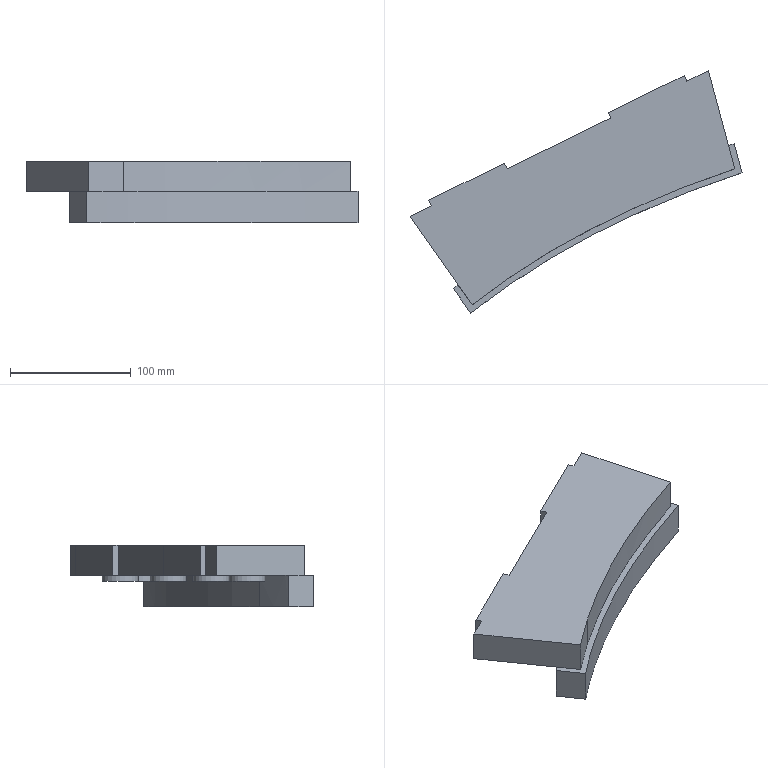Part | NX | features solid 2 | 1 solid | 33 faces | box 275.465 x 201.523 x 51 mm | volume 719217 mm3 | plane 23 | spline 5 | cylinder 5 | commonest cylinder face diameters 30 x5
STEP:
#1=CARTESIAN_POINT('',(-429.757,480.324,20.));
#2=VERTEX_POINT('',#1);
#3=CARTESIAN_POINT('',(-414.757,480.324,20.));
#4=DIRECTION('',(0.,0.,-1.));
#5=DIRECTION('',(-1.,0.,0.));
#6=AXIS2_PLACEMENT_3D('',#3,#4,#5);
#7=CIRCLE('',#6,15.);
#8=EDGE_CURVE('',#2,#2,#7,.F.);
#9=ORIENTED_EDGE('',*,*,#8,.T.);
#10=EDGE_LOOP('',(#9));
#11=FACE_BOUND('',#10,.T.);
#12=CARTESIAN_POINT('',(-459.757,495.324,20.));
#13=VERTEX_POINT('',#12);
#14=CARTESIAN_POINT('',(-444.757,495.324,20.));
#15=DIRECTION('',(0.,0.,-1.));
#16=DIRECTION('',(-1.,0.,0.));
#17=AXIS2_PLACEMENT_3D('',#14,#15,#16);
#18=CIRCLE('',#17,15.);
#19=EDGE_CURVE('',#13,#13,#18,.F.);
#20=ORIENTED_EDGE('',*,*,#19,.T.);
#21=EDGE_LOOP('',(#20));
#22=FACE_BOUND('',#21,.T.);
#23=CARTESIAN_POINT('',(-514.757,455.324,20.));
#24=VERTEX_POINT('',#23);
#25=CARTESIAN_POINT('',(-499.757,455.324,20.));
#26=DIRECTION('',(0.,0.,-1.));
#27=DIRECTION('',(-1.,0.,0.));
#28=AXIS2_PLACEMENT_3D('',#25,#26,#27);
#29=CIRCLE('',#28,15.);
#30=EDGE_CURVE('',#24,#24,#29,.F.);
#31=ORIENTED_EDGE('',*,*,#30,.T.);
#32=EDGE_LOOP('',(#31));
#33=FACE_BOUND('',#32,.T.);
#34=CARTESIAN_POINT('',(-609.757,390.324,20.));
#35=VERTEX_POINT('',#34);
#36=CARTESIAN_POINT('',(-594.757,390.324,20.));
#37=DIRECTION('',(0.,0.,-1.));
#38=DIRECTION('',(-1.,0.,0.));
#39=AXIS2_PLACEMENT_3D('',#36,#37,#38);
#40=CIRCLE('',#39,15.);
#41=EDGE_CURVE('',#35,#35,#40,.F.);
#42=ORIENTED_EDGE('',*,*,#41,.T.);
#43=EDGE_LOOP('',(#42));
#44=FACE_BOUND('',#43,.T.);
#45=CARTESIAN_POINT('',(-599.757,420.324,20.));
#46=VERTEX_POINT('',#45);
#47=CARTESIAN_POINT('',(-584.757,420.324,20.));
#48=DIRECTION('',(0.,0.,-1.));
#49=DIRECTION('',(-1.,0.,0.));
#50=AXIS2_PLACEMENT_3D('',#47,#48,#49);
#51=CIRCLE('',#50,15.);
#52=EDGE_CURVE('',#46,#46,#51,.F.);
#53=ORIENTED_EDGE('',*,*,#52,.T.);
#54=EDGE_LOOP('',(#53));
#55=FACE_BOUND('',#54,.T.);
#56=CARTESIAN_POINT('',(-605.432,358.634,20.));
#57=VERTEX_POINT('',#56);
#58=CARTESIAN_POINT('',(-645.465,415.808,20.));
#59=VERTEX_POINT('',#58);
#60=CARTESIAN_POINT('',(-593.778,341.99,20.));
#61=DIRECTION('',(0.5736,-0.8192,0.));
#62=VECTOR('',#61,1000.);
#63=LINE('',#60,#62);
#64=EDGE_CURVE('',#57,#59,#63,.F.);
#65=ORIENTED_EDGE('',*,*,#64,.T.);
#66=CARTESIAN_POINT('',(-627.838,424.405,20.));
#67=VERTEX_POINT('',#66);
#68=CARTESIAN_POINT('',(-664.162,406.689,20.));
#69=DIRECTION('',(-0.8988,-0.4384,0.));
#70=VECTOR('',#69,1000.);
#71=LINE('',#68,#70);
#72=EDGE_CURVE('',#59,#67,#71,.F.);
#73=ORIENTED_EDGE('',*,*,#72,.T.);
#74=CARTESIAN_POINT('',(-630.03,428.899,20.));
#75=VERTEX_POINT('',#74);
#76=CARTESIAN_POINT('',(-589.593,345.992,20.));
#77=DIRECTION('',(0.4384,-0.8988,0.));
#78=VECTOR('',#77,1000.);
#79=LINE('',#76,#78);
#80=EDGE_CURVE('',#67,#75,#79,.F.);
#81=ORIENTED_EDGE('',*,*,#80,.T.);
#82=CARTESIAN_POINT('',(-567.114,459.585,20.));
#83=VERTEX_POINT('',#82);
#84=CARTESIAN_POINT('',(-621.042,433.283,20.));
#85=DIRECTION('',(0.8988,0.4384,0.));
#86=VECTOR('',#85,1000.);
#87=LINE('',#84,#86);
#88=EDGE_CURVE('',#75,#83,#87,.T.);
#89=ORIENTED_EDGE('',*,*,#88,.T.);
#90=CARTESIAN_POINT('',(-564.922,455.091,20.));
#91=VERTEX_POINT('',#90);
#92=CARTESIAN_POINT('',(-526.677,376.678,20.));
#93=DIRECTION('',(0.4384,-0.8988,0.));
#94=VECTOR('',#93,1000.);
#95=LINE('',#92,#94);
#96=EDGE_CURVE('',#91,#83,#95,.F.);
#97=ORIENTED_EDGE('',*,*,#96,.F.);
#98=CARTESIAN_POINT('',(-478.788,497.102,20.));
#99=VERTEX_POINT('',#98);
#100=CARTESIAN_POINT('',(-664.162,406.689,20.));
#101=DIRECTION('',(-0.8988,-0.4384,0.));
#102=VECTOR('',#101,1000.);
#103=LINE('',#100,#102);
#104=EDGE_CURVE('',#91,#99,#103,.F.);
#105=ORIENTED_EDGE('',*,*,#104,.T.);
#106=CARTESIAN_POINT('',(-480.98,501.596,20.));
#107=VERTEX_POINT('',#106);
#108=CARTESIAN_POINT('',(-440.543,418.688,20.));
#109=DIRECTION('',(0.4384,-0.8988,0.));
#110=VECTOR('',#109,1000.);
#111=LINE('',#108,#110);
#112=EDGE_CURVE('',#99,#107,#111,.F.);
#113=ORIENTED_EDGE('',*,*,#112,.T.);
#114=CARTESIAN_POINT('',(-418.064,532.282,20.));
#115=VERTEX_POINT('',#114);
#116=CARTESIAN_POINT('',(-391.1,545.433,20.));
#117=DIRECTION('',(0.8988,0.4384,0.));
#118=VECTOR('',#117,1000.);
#119=LINE('',#116,#118);
#120=EDGE_CURVE('',#107,#115,#119,.T.);
#121=ORIENTED_EDGE('',*,*,#120,.T.);
#122=CARTESIAN_POINT('',(-415.872,527.788,20.));
#123=VERTEX_POINT('',#122);
#124=CARTESIAN_POINT('',(-377.627,449.374,20.));
#125=DIRECTION('',(0.4384,-0.8988,0.));
#126=VECTOR('',#125,1000.);
#127=LINE('',#124,#126);
#128=EDGE_CURVE('',#123,#115,#127,.F.);
#129=ORIENTED_EDGE('',*,*,#128,.F.);
#130=CARTESIAN_POINT('',(-397.924,536.542,20.));
#131=VERTEX_POINT('',#130);
#132=CARTESIAN_POINT('',(-664.162,406.689,20.));
#133=DIRECTION('',(-0.8988,-0.4384,0.));
#134=VECTOR('',#133,1000.);
#135=LINE('',#132,#134);
#136=EDGE_CURVE('',#123,#131,#135,.F.);
#137=ORIENTED_EDGE('',*,*,#136,.T.);
#138=CARTESIAN_POINT('',(-381.238,474.267,20.));
#139=VERTEX_POINT('',#138);
#140=CARTESIAN_POINT('',(-381.309,474.533,20.));
#141=DIRECTION('',(0.2588,-0.9659,0.));
#142=VECTOR('',#141,1000.);
#143=LINE('',#140,#142);
#144=EDGE_CURVE('',#131,#139,#143,.T.);
#145=ORIENTED_EDGE('',*,*,#144,.T.);
#146=CARTESIAN_POINT('',(-575.957,380.187,20.));
#147=VERTEX_POINT('',#146);
#148=CARTESIAN_POINT('',(-575.957,380.187,20.));
#149=CARTESIAN_POINT('',(-546.051,400.694,20.));
#150=CARTESIAN_POINT('',(-498.952,427.295,20.));
#151=CARTESIAN_POINT('',(-432.464,456.265,20.));
#152=CARTESIAN_POINT('',(-398.428,468.585,20.));
#153=CARTESIAN_POINT('',(-381.238,474.267,20.));
#154=B_SPLINE_CURVE_WITH_KNOTS('',3,(#148,#149,#150,#151,#152,#153),.UNSPECIFIED.,.F.,.F.,(4,1,1,4),(0.4449,0.5537,0.6081,0.6625),.UNSPECIFIED.);
#155=EDGE_CURVE('',#147,#139,#154,.T.);
#156=ORIENTED_EDGE('',*,*,#155,.F.);
#157=CARTESIAN_POINT('',(-575.957,380.187,20.));
#158=VERTEX_POINT('',#157);
#159=CARTESIAN_POINT('',(-564.773,363.606,20.));
#160=DIRECTION('',(0.5592,-0.829,0.));
#161=VECTOR('',#160,1000.);
#162=LINE('',#159,#161);
#163=EDGE_CURVE('',#147,#158,#162,.F.);
#164=ORIENTED_EDGE('',*,*,#163,.T.);
#165=CARTESIAN_POINT('',(-575.957,380.187,20.));
#166=CARTESIAN_POINT('',(-586.035,373.272,20.));
#167=CARTESIAN_POINT('',(-595.868,366.096,20.));
#168=CARTESIAN_POINT('',(-605.432,358.634,20.));
#169=B_SPLINE_CURVE_WITH_KNOTS('',3,(#165,#166,#167,#168),.UNSPECIFIED.,.F.,.F.,(4,4),(0.8565,0.8932),.UNSPECIFIED.);
#170=EDGE_CURVE('',#57,#158,#169,.F.);
#171=ORIENTED_EDGE('',*,*,#170,.F.);
#172=EDGE_LOOP('',(#65,#73,#81,#89,#97,#105,#113,#121,#129,#137,#145,#156,#164,#171));
#173=FACE_BOUND('',#172,.T.);
#174=CARTESIAN_POINT('',(-561.977,359.461,20.));
#175=DIRECTION('',(0.,0.,-1.));
#176=DIRECTION('',(-1.,0.,0.));
#177=AXIS2_PLACEMENT_3D('',#174,#175,#176);
#178=PLANE('',#177);
#179=ADVANCED_FACE('',(#11,#22,#33,#44,#55,#173),#178,.T.);
#180=CARTESIAN_POINT('',(-593.945,342.229,20.));
#181=VERTEX_POINT('',#180);
#182=CARTESIAN_POINT('',(-593.945,342.229,45.));
#183=VERTEX_POINT('',#182);
#184=CARTESIAN_POINT('',(-593.945,342.229,32.5));
#185=DIRECTION('',(0.,0.,-1.));
#186=VECTOR('',#185,1000.);
#187=LINE('',#184,#186);
#188=EDGE_CURVE('',#181,#183,#187,.F.);
#189=ORIENTED_EDGE('',*,*,#188,.F.);
#190=CARTESIAN_POINT('',(-564.773,363.606,20.));
#191=VERTEX_POINT('',#190);
#192=CARTESIAN_POINT('',(-564.773,363.606,20.));
#193=CARTESIAN_POINT('',(-574.716,356.784,20.));
#194=CARTESIAN_POINT('',(-584.447,349.668,20.));
#195=CARTESIAN_POINT('',(-593.945,342.229,20.));
#196=B_SPLINE_CURVE_WITH_KNOTS('',3,(#192,#193,#194,#195),.UNSPECIFIED.,.F.,.F.,(4,4),(0.7865,0.8227),.UNSPECIFIED.);
#197=EDGE_CURVE('',#181,#191,#196,.F.);
#198=ORIENTED_EDGE('',*,*,#197,.T.);
#199=CARTESIAN_POINT('',(-564.773,363.606,45.));
#200=VERTEX_POINT('',#199);
#201=CARTESIAN_POINT('',(-564.773,363.606,32.5));
#202=DIRECTION('',(0.,0.,-1.));
#203=VECTOR('',#202,1000.);
#204=LINE('',#201,#203);
#205=EDGE_CURVE('',#191,#200,#204,.F.);
#206=ORIENTED_EDGE('',*,*,#205,.T.);
#207=CARTESIAN_POINT('',(-593.945,342.229,45.));
#208=CARTESIAN_POINT('',(-584.456,349.661,45.));
#209=CARTESIAN_POINT('',(-574.725,356.777,45.));
#210=CARTESIAN_POINT('',(-564.773,363.606,45.));
#211=B_SPLINE_CURVE_WITH_KNOTS('',3,(#207,#208,#209,#210),.UNSPECIFIED.,.F.,.F.,(4,4),(0.3243,0.3606),.UNSPECIFIED.);
#212=EDGE_CURVE('',#183,#200,#211,.T.);
#213=ORIENTED_EDGE('',*,*,#212,.F.);
#214=EDGE_LOOP('',(#189,#198,#206,#213));
#215=FACE_BOUND('',#214,.T.);
#216=CARTESIAN_POINT('',(-593.945,342.229,45.));
#217=CARTESIAN_POINT('',(-593.945,342.229,20.));
#218=CARTESIAN_POINT('',(-589.197,345.947,45.));
#219=CARTESIAN_POINT('',(-589.197,345.947,20.));
#220=CARTESIAN_POINT('',(-579.602,353.212,45.));
#221=CARTESIAN_POINT('',(-579.602,353.212,20.));
#222=CARTESIAN_POINT('',(-569.701,360.225,45.));
#223=CARTESIAN_POINT('',(-569.701,360.225,20.));
#224=CARTESIAN_POINT('',(-564.773,363.606,45.));
#225=CARTESIAN_POINT('',(-564.773,363.606,20.));
#226=B_SPLINE_SURFACE_WITH_KNOTS('',3,1,((#216,#217),(#218,#219),(#220,#221),(#222,#223),(#224,#225)),.SURF_OF_LINEAR_EXTRUSION.,.F.,.F.,.F.,(4,1,4),(2,2),(0.8993,0.9497,1.),(0.,1.),.UNSPECIFIED.);
#227=ADVANCED_FACE('',(#215),#226,.F.);
#228=CARTESIAN_POINT('',(-645.465,415.808,45.));
#229=VERTEX_POINT('',#228);
#230=CARTESIAN_POINT('',(-627.838,424.405,45.));
#231=VERTEX_POINT('',#230);
#232=CARTESIAN_POINT('',(-664.162,406.689,45.));
#233=DIRECTION('',(0.8988,0.4384,0.));
#234=VECTOR('',#233,1000.);
#235=LINE('',#232,#234);
#236=EDGE_CURVE('',#229,#231,#235,.T.);
#237=ORIENTED_EDGE('',*,*,#236,.F.);
#238=CARTESIAN_POINT('',(-593.778,341.99,45.));
#239=DIRECTION('',(0.5736,-0.8192,0.));
#240=VECTOR('',#239,1000.);
#241=LINE('',#238,#240);
#242=EDGE_CURVE('',#183,#229,#241,.F.);
#243=ORIENTED_EDGE('',*,*,#242,.F.);
#244=ORIENTED_EDGE('',*,*,#212,.T.);
#245=CARTESIAN_POINT('',(-376.053,454.916,45.));
#246=VERTEX_POINT('',#245);
#247=CARTESIAN_POINT('',(-564.773,363.606,45.));
#248=CARTESIAN_POINT('',(-535.83,383.463,45.));
#249=CARTESIAN_POINT('',(-474.62,418.047,45.));
#250=CARTESIAN_POINT('',(-409.268,443.891,45.));
#251=CARTESIAN_POINT('',(-376.053,454.916,45.));
#252=B_SPLINE_CURVE_WITH_KNOTS('',3,(#247,#248,#249,#250,#251),.UNSPECIFIED.,.F.,.F.,(4,1,4),(-0.004993,0.1002,0.2053),.UNSPECIFIED.);
#253=EDGE_CURVE('',#200,#246,#252,.T.);
#254=ORIENTED_EDGE('',*,*,#253,.T.);
#255=CARTESIAN_POINT('',(-397.924,536.542,45.));
#256=VERTEX_POINT('',#255);
#257=CARTESIAN_POINT('',(-381.309,474.533,45.));
#258=DIRECTION('',(0.2588,-0.9659,0.));
#259=VECTOR('',#258,1000.);
#260=LINE('',#257,#259);
#261=EDGE_CURVE('',#256,#246,#260,.T.);
#262=ORIENTED_EDGE('',*,*,#261,.F.);
#263=CARTESIAN_POINT('',(-415.872,527.788,45.));
#264=VERTEX_POINT('',#263);
#265=CARTESIAN_POINT('',(-664.162,406.689,45.));
#266=DIRECTION('',(0.8988,0.4384,0.));
#267=VECTOR('',#266,1000.);
#268=LINE('',#265,#267);
#269=EDGE_CURVE('',#264,#256,#268,.T.);
#270=ORIENTED_EDGE('',*,*,#269,.F.);
#271=CARTESIAN_POINT('',(-418.064,532.282,45.));
#272=VERTEX_POINT('',#271);
#273=CARTESIAN_POINT('',(169.825,-673.069,45.));
#274=DIRECTION('',(-0.4384,0.8988,0.));
#275=VECTOR('',#274,1000.);
#276=LINE('',#273,#275);
#277=EDGE_CURVE('',#264,#272,#276,.T.);
#278=ORIENTED_EDGE('',*,*,#277,.T.);
#279=CARTESIAN_POINT('',(-480.98,501.596,45.));
#280=VERTEX_POINT('',#279);
#281=CARTESIAN_POINT('',(-391.1,545.433,45.));
#282=DIRECTION('',(0.8988,0.4384,0.));
#283=VECTOR('',#282,1000.);
#284=LINE('',#281,#283);
#285=EDGE_CURVE('',#280,#272,#284,.T.);
#286=ORIENTED_EDGE('',*,*,#285,.F.);
#287=CARTESIAN_POINT('',(-478.788,497.102,45.));
#288=VERTEX_POINT('',#287);
#289=CARTESIAN_POINT('',(106.909,-703.754,45.));
#290=DIRECTION('',(-0.4384,0.8988,0.));
#291=VECTOR('',#290,1000.);
#292=LINE('',#289,#291);
#293=EDGE_CURVE('',#288,#280,#292,.T.);
#294=ORIENTED_EDGE('',*,*,#293,.F.);
#295=CARTESIAN_POINT('',(-564.922,455.091,45.));
#296=VERTEX_POINT('',#295);
#297=CARTESIAN_POINT('',(-664.162,406.689,45.));
#298=DIRECTION('',(0.8988,0.4384,0.));
#299=VECTOR('',#298,1000.);
#300=LINE('',#297,#299);
#301=EDGE_CURVE('',#296,#288,#300,.T.);
#302=ORIENTED_EDGE('',*,*,#301,.F.);
#303=CARTESIAN_POINT('',(-567.114,459.585,45.));
#304=VERTEX_POINT('',#303);
#305=CARTESIAN_POINT('',(20.775,-745.765,45.));
#306=DIRECTION('',(-0.4384,0.8988,0.));
#307=VECTOR('',#306,1000.);
#308=LINE('',#305,#307);
#309=EDGE_CURVE('',#296,#304,#308,.T.);
#310=ORIENTED_EDGE('',*,*,#309,.T.);
#311=CARTESIAN_POINT('',(-630.03,428.899,45.));
#312=VERTEX_POINT('',#311);
#313=CARTESIAN_POINT('',(-621.042,433.283,45.));
#314=DIRECTION('',(0.8988,0.4384,0.));
#315=VECTOR('',#314,1000.);
#316=LINE('',#313,#315);
#317=EDGE_CURVE('',#312,#304,#316,.T.);
#318=ORIENTED_EDGE('',*,*,#317,.F.);
#319=CARTESIAN_POINT('',(-42.141,-776.451,45.));
#320=DIRECTION('',(-0.4384,0.8988,0.));
#321=VECTOR('',#320,1000.);
#322=LINE('',#319,#321);
#323=EDGE_CURVE('',#231,#312,#322,.T.);
#324=ORIENTED_EDGE('',*,*,#323,.F.);
#325=EDGE_LOOP('',(#237,#243,#244,#254,#262,#270,#278,#286,#294,#302,#310,#318,#324));
#326=FACE_BOUND('',#325,.T.);
#327=CARTESIAN_POINT('',(-80.139,-794.984,45.));
#328=DIRECTION('',(0.,0.,1.));
#329=DIRECTION('',(1.,0.,0.));
#330=AXIS2_PLACEMENT_3D('',#327,#328,#329);
#331=PLANE('',#330);
#332=ADVANCED_FACE('',(#326),#331,.T.);
#333=ORIENTED_EDGE('',*,*,#72,.F.);
#334=CARTESIAN_POINT('',(-645.465,415.808,70.));
#335=DIRECTION('',(0.,0.,1.));
#336=VECTOR('',#335,1000.);
#337=LINE('',#334,#336);
#338=EDGE_CURVE('',#59,#229,#337,.T.);
#339=ORIENTED_EDGE('',*,*,#338,.T.);
#340=ORIENTED_EDGE('',*,*,#236,.T.);
#341=CARTESIAN_POINT('',(-627.838,424.405,70.));
#342=DIRECTION('',(0.,0.,-1.));
#343=VECTOR('',#342,1000.);
#344=LINE('',#341,#343);
#345=EDGE_CURVE('',#231,#67,#344,.T.);
#346=ORIENTED_EDGE('',*,*,#345,.T.);
#347=EDGE_LOOP('',(#333,#339,#340,#346));
#348=FACE_BOUND('',#347,.T.);
#349=CARTESIAN_POINT('',(-664.162,406.689,70.));
#350=DIRECTION('',(-0.4384,0.8988,0.));
#351=DIRECTION('',(-0.8988,-0.4384,0.));
#352=AXIS2_PLACEMENT_3D('',#349,#350,#351);
#353=PLANE('',#352);
#354=ADVANCED_FACE('',(#348),#353,.T.);
#355=CARTESIAN_POINT('',(-376.48,475.827,20.));
#356=VERTEX_POINT('',#355);
#357=CARTESIAN_POINT('',(-376.48,475.827,-6.));
#358=VERTEX_POINT('',#357);
#359=CARTESIAN_POINT('',(-376.48,475.827,7.));
#360=DIRECTION('',(0.,0.,1.));
#361=VECTOR('',#360,1000.);
#362=LINE('',#359,#361);
#363=EDGE_CURVE('',#356,#358,#362,.F.);
#364=ORIENTED_EDGE('',*,*,#363,.F.);
#365=CARTESIAN_POINT('',(-370.,451.645,20.));
#366=VERTEX_POINT('',#365);
#367=CARTESIAN_POINT('',(-359.814,413.63,20.));
#368=DIRECTION('',(0.2588,-0.9659,0.));
#369=VECTOR('',#368,1000.);
#370=LINE('',#367,#369);
#371=EDGE_CURVE('',#366,#356,#370,.F.);
#372=ORIENTED_EDGE('',*,*,#371,.F.);
#373=CARTESIAN_POINT('',(-370.,451.645,-6.));
#374=VERTEX_POINT('',#373);
#375=CARTESIAN_POINT('',(-370.,451.645,7.));
#376=DIRECTION('',(0.,0.,-1.));
#377=VECTOR('',#376,1000.);
#378=LINE('',#375,#377);
#379=EDGE_CURVE('',#374,#366,#378,.F.);
#380=ORIENTED_EDGE('',*,*,#379,.F.);
#381=CARTESIAN_POINT('',(-38.926,-783.941,-6.));
#382=DIRECTION('',(0.2588,-0.9659,0.));
#383=VECTOR('',#382,1000.);
#384=LINE('',#381,#383);
#385=EDGE_CURVE('',#358,#374,#384,.T.);
#386=ORIENTED_EDGE('',*,*,#385,.F.);
#387=EDGE_LOOP('',(#364,#372,#380,#386));
#388=FACE_BOUND('',#387,.T.);
#389=CARTESIAN_POINT('',(-409.752,600.,0.));
#390=DIRECTION('',(-0.9659,-0.2588,0.));
#391=DIRECTION('',(0.2588,-0.9659,0.));
#392=AXIS2_PLACEMENT_3D('',#389,#390,#391);
#393=PLANE('',#392);
#394=ADVANCED_FACE('',(#388),#393,.F.);
#395=ORIENTED_EDGE('',*,*,#155,.T.);
#396=CARTESIAN_POINT('',(-381.238,474.267,20.));
#397=CARTESIAN_POINT('',(-379.653,474.791,20.));
#398=CARTESIAN_POINT('',(-378.067,475.311,20.));
#399=CARTESIAN_POINT('',(-376.48,475.827,20.));
#400=B_SPLINE_CURVE_WITH_KNOTS('',3,(#396,#397,#398,#399),.UNSPECIFIED.,.F.,.F.,(4,4),(0.7627,0.7804),.UNSPECIFIED.);
#401=EDGE_CURVE('',#139,#356,#400,.T.);
#402=ORIENTED_EDGE('',*,*,#401,.T.);
#403=ORIENTED_EDGE('',*,*,#363,.T.);
#404=CARTESIAN_POINT('',(-575.957,380.187,-6.));
#405=VERTEX_POINT('',#404);
#406=CARTESIAN_POINT('',(-575.957,380.187,-6.));
#407=CARTESIAN_POINT('',(-545.364,401.165,-6.));
#408=CARTESIAN_POINT('',(-497.124,428.288,-6.));
#409=CARTESIAN_POINT('',(-428.974,457.67,-6.));
#410=CARTESIAN_POINT('',(-394.098,470.103,-6.));
#411=CARTESIAN_POINT('',(-376.48,475.827,-6.));
#412=B_SPLINE_CURVE_WITH_KNOTS('',3,(#406,#407,#408,#409,#410,#411),.UNSPECIFIED.,.F.,.F.,(4,1,1,4),(0.4454,0.5567,0.6123,0.6679),.UNSPECIFIED.);
#413=EDGE_CURVE('',#405,#358,#412,.T.);
#414=ORIENTED_EDGE('',*,*,#413,.F.);
#415=CARTESIAN_POINT('',(-575.957,380.187,9.5));
#416=DIRECTION('',(0.,0.,1.));
#417=VECTOR('',#416,1000.);
#418=LINE('',#415,#417);
#419=EDGE_CURVE('',#405,#147,#418,.T.);
#420=ORIENTED_EDGE('',*,*,#419,.T.);
#421=EDGE_LOOP('',(#395,#402,#403,#414,#420));
#422=FACE_BOUND('',#421,.T.);
#423=CARTESIAN_POINT('',(-575.957,380.187,-6.));
#424=CARTESIAN_POINT('',(-575.957,380.187,20.));
#425=CARTESIAN_POINT('',(-545.186,401.287,-6.));
#426=CARTESIAN_POINT('',(-545.186,401.287,20.));
#427=CARTESIAN_POINT('',(-480.278,437.706,-6.));
#428=CARTESIAN_POINT('',(-480.278,437.706,20.));
#429=CARTESIAN_POINT('',(-411.43,464.473,-6.));
#430=CARTESIAN_POINT('',(-411.43,464.473,20.));
#431=CARTESIAN_POINT('',(-376.48,475.827,-6.));
#432=CARTESIAN_POINT('',(-376.48,475.827,20.));
#433=B_SPLINE_SURFACE_WITH_KNOTS('',3,1,((#423,#424),(#425,#426),(#427,#428),(#429,#430),(#431,#432)),.SURF_OF_LINEAR_EXTRUSION.,.F.,.F.,.F.,(4,1,4),(2,2),(0.0006942,0.3906,0.7804),(0.,1.),.UNSPECIFIED.);
#434=ADVANCED_FACE('',(#422),#433,.F.);
#435=CARTESIAN_POINT('',(-376.053,454.916,20.));
#436=VERTEX_POINT('',#435);
#437=CARTESIAN_POINT('',(-381.309,474.533,20.));
#438=DIRECTION('',(0.2588,-0.9659,0.));
#439=VECTOR('',#438,1000.);
#440=LINE('',#437,#439);
#441=EDGE_CURVE('',#139,#436,#440,.T.);
#442=ORIENTED_EDGE('',*,*,#441,.F.);
#443=ORIENTED_EDGE('',*,*,#144,.F.);
#444=CARTESIAN_POINT('',(-397.924,536.542,70.));
#445=DIRECTION('',(0.,0.,1.));
#446=VECTOR('',#445,1000.);
#447=LINE('',#444,#446);
#448=EDGE_CURVE('',#131,#256,#447,.T.);
#449=ORIENTED_EDGE('',*,*,#448,.T.);
#450=ORIENTED_EDGE('',*,*,#261,.T.);
#451=CARTESIAN_POINT('',(-376.053,454.916,32.5));
#452=DIRECTION('',(0.,0.,-1.));
#453=VECTOR('',#452,1000.);
#454=LINE('',#451,#453);
#455=EDGE_CURVE('',#436,#246,#454,.F.);
#456=ORIENTED_EDGE('',*,*,#455,.F.);
#457=EDGE_LOOP('',(#442,#443,#449,#450,#456));
#458=FACE_BOUND('',#457,.T.);
#459=CARTESIAN_POINT('',(-381.309,474.533,20.));
#460=DIRECTION('',(-0.9659,-0.2588,0.));
#461=DIRECTION('',(0.2588,-0.9659,0.));
#462=AXIS2_PLACEMENT_3D('',#459,#460,#461);
#463=PLANE('',#462);
#464=ADVANCED_FACE('',(#458),#463,.F.);
#465=ORIENTED_EDGE('',*,*,#448,.F.);
#466=ORIENTED_EDGE('',*,*,#136,.F.);
#467=CARTESIAN_POINT('',(-415.872,527.788,70.));
#468=DIRECTION('',(0.,0.,-1.));
#469=VECTOR('',#468,1000.);
#470=LINE('',#467,#469);
#471=EDGE_CURVE('',#264,#123,#470,.T.);
#472=ORIENTED_EDGE('',*,*,#471,.F.);
#473=ORIENTED_EDGE('',*,*,#269,.T.);
#474=EDGE_LOOP('',(#465,#466,#472,#473));
#475=FACE_BOUND('',#474,.T.);
#476=CARTESIAN_POINT('',(-664.162,406.689,70.));
#477=DIRECTION('',(-0.4384,0.8988,0.));
#478=DIRECTION('',(-0.8988,-0.4384,0.));
#479=AXIS2_PLACEMENT_3D('',#476,#477,#478);
#480=PLANE('',#479);
#481=ADVANCED_FACE('',(#475),#480,.T.);
#482=CARTESIAN_POINT('',(-418.064,532.282,45.));
#483=DIRECTION('',(0.,0.,-1.));
#484=VECTOR('',#483,1000.);
#485=LINE('',#482,#484);
#486=EDGE_CURVE('',#272,#115,#485,.T.);
#487=ORIENTED_EDGE('',*,*,#486,.F.);
#488=ORIENTED_EDGE('',*,*,#277,.F.);
#489=ORIENTED_EDGE('',*,*,#471,.T.);
#490=ORIENTED_EDGE('',*,*,#128,.T.);
#491=EDGE_LOOP('',(#487,#488,#489,#490));
#492=FACE_BOUND('',#491,.T.);
#493=CARTESIAN_POINT('',(-415.872,527.788,45.));
#494=DIRECTION('',(0.8988,0.4384,0.));
#495=DIRECTION('',(-0.4384,0.8988,0.));
#496=AXIS2_PLACEMENT_3D('',#493,#494,#495);
#497=PLANE('',#496);
#498=ADVANCED_FACE('',(#492),#497,.T.);
#499=ORIENTED_EDGE('',*,*,#486,.T.);
#500=ORIENTED_EDGE('',*,*,#120,.F.);
#501=CARTESIAN_POINT('',(-480.98,501.596,45.));
#502=DIRECTION('',(0.,0.,-1.));
#503=VECTOR('',#502,1000.);
#504=LINE('',#501,#503);
#505=EDGE_CURVE('',#280,#107,#504,.T.);
#506=ORIENTED_EDGE('',*,*,#505,.F.);
#507=ORIENTED_EDGE('',*,*,#285,.T.);
#508=EDGE_LOOP('',(#499,#500,#506,#507));
#509=FACE_BOUND('',#508,.T.);
#510=CARTESIAN_POINT('',(-391.1,545.433,45.));
#511=DIRECTION('',(0.4384,-0.8988,0.));
#512=DIRECTION('',(0.,0.,-1.));
#513=AXIS2_PLACEMENT_3D('',#510,#511,#512);
#514=PLANE('',#513);
#515=ADVANCED_FACE('',(#509),#514,.F.);
#516=ORIENTED_EDGE('',*,*,#505,.T.);
#517=ORIENTED_EDGE('',*,*,#112,.F.);
#518=CARTESIAN_POINT('',(-478.788,497.102,70.));
#519=DIRECTION('',(0.,0.,-1.));
#520=VECTOR('',#519,1000.);
#521=LINE('',#518,#520);
#522=EDGE_CURVE('',#288,#99,#521,.T.);
#523=ORIENTED_EDGE('',*,*,#522,.F.);
#524=ORIENTED_EDGE('',*,*,#293,.T.);
#525=EDGE_LOOP('',(#516,#517,#523,#524));
#526=FACE_BOUND('',#525,.T.);
#527=CARTESIAN_POINT('',(-478.788,497.102,45.));
#528=DIRECTION('',(0.8988,0.4384,0.));
#529=DIRECTION('',(-0.4384,0.8988,0.));
#530=AXIS2_PLACEMENT_3D('',#527,#528,#529);
#531=PLANE('',#530);
#532=ADVANCED_FACE('',(#526),#531,.F.);
#533=ORIENTED_EDGE('',*,*,#301,.T.);
#534=ORIENTED_EDGE('',*,*,#522,.T.);
#535=ORIENTED_EDGE('',*,*,#104,.F.);
#536=CARTESIAN_POINT('',(-564.922,455.091,70.));
#537=DIRECTION('',(0.,0.,-1.));
#538=VECTOR('',#537,1000.);
#539=LINE('',#536,#538);
#540=EDGE_CURVE('',#296,#91,#539,.T.);
#541=ORIENTED_EDGE('',*,*,#540,.F.);
#542=EDGE_LOOP('',(#533,#534,#535,#541));
#543=FACE_BOUND('',#542,.T.);
#544=CARTESIAN_POINT('',(-664.162,406.689,70.));
#545=DIRECTION('',(-0.4384,0.8988,0.));
#546=DIRECTION('',(-0.8988,-0.4384,0.));
#547=AXIS2_PLACEMENT_3D('',#544,#545,#546);
#548=PLANE('',#547);
#549=ADVANCED_FACE('',(#543),#548,.T.);
#550=CARTESIAN_POINT('',(-567.114,459.585,45.));
#551=DIRECTION('',(0.,0.,-1.));
#552=VECTOR('',#551,1000.);
#553=LINE('',#550,#552);
#554=EDGE_CURVE('',#304,#83,#553,.T.);
#555=ORIENTED_EDGE('',*,*,#554,.F.);
#556=ORIENTED_EDGE('',*,*,#309,.F.);
#557=ORIENTED_EDGE('',*,*,#540,.T.);
#558=ORIENTED_EDGE('',*,*,#96,.T.);
#559=EDGE_LOOP('',(#555,#556,#557,#558));
#560=FACE_BOUND('',#559,.T.);
#561=CARTESIAN_POINT('',(-564.922,455.091,45.));
#562=DIRECTION('',(0.8988,0.4384,0.));
#563=DIRECTION('',(-0.4384,0.8988,0.));
#564=AXIS2_PLACEMENT_3D('',#561,#562,#563);
#565=PLANE('',#564);
#566=ADVANCED_FACE('',(#560),#565,.T.);
#567=ORIENTED_EDGE('',*,*,#554,.T.);
#568=ORIENTED_EDGE('',*,*,#88,.F.);
#569=CARTESIAN_POINT('',(-630.03,428.899,45.));
#570=DIRECTION('',(0.,0.,-1.));
#571=VECTOR('',#570,1000.);
#572=LINE('',#569,#571);
#573=EDGE_CURVE('',#312,#75,#572,.T.);
#574=ORIENTED_EDGE('',*,*,#573,.F.);
#575=ORIENTED_EDGE('',*,*,#317,.T.);
#576=EDGE_LOOP('',(#567,#568,#574,#575));
#577=FACE_BOUND('',#576,.T.);
#578=CARTESIAN_POINT('',(-621.042,433.283,45.));
#579=DIRECTION('',(0.4384,-0.8988,0.));
#580=DIRECTION('',(0.,0.,-1.));
#581=AXIS2_PLACEMENT_3D('',#578,#579,#580);
#582=PLANE('',#581);
#583=ADVANCED_FACE('',(#577),#582,.F.);
#584=ORIENTED_EDGE('',*,*,#573,.T.);
#585=ORIENTED_EDGE('',*,*,#80,.F.);
#586=ORIENTED_EDGE('',*,*,#345,.F.);
#587=ORIENTED_EDGE('',*,*,#323,.T.);
#588=EDGE_LOOP('',(#584,#585,#586,#587));
#589=FACE_BOUND('',#588,.T.);
#590=CARTESIAN_POINT('',(-627.838,424.405,45.));
#591=DIRECTION('',(0.8988,0.4384,0.));
#592=DIRECTION('',(-0.4384,0.8988,0.));
#593=AXIS2_PLACEMENT_3D('',#590,#591,#592);
#594=PLANE('',#593);
#595=ADVANCED_FACE('',(#589),#594,.F.);
#596=ORIENTED_EDGE('',*,*,#163,.F.);
#597=ORIENTED_EDGE('',*,*,#419,.F.);
#598=CARTESIAN_POINT('',(-575.957,380.187,-6.));
#599=VERTEX_POINT('',#598);
#600=CARTESIAN_POINT('',(826.517,-1699.065,-6.));
#601=DIRECTION('',(-0.5592,0.829,0.));
#602=VECTOR('',#601,1000.);
#603=LINE('',#600,#602);
#604=EDGE_CURVE('',#405,#599,#603,.T.);
#605=ORIENTED_EDGE('',*,*,#604,.T.);
#606=CARTESIAN_POINT('',(-575.957,380.187,20.003));
#607=DIRECTION('',(0.,0.,1.));
#608=VECTOR('',#607,1000.);
#609=LINE('',#606,#608);
#610=EDGE_CURVE('',#599,#158,#609,.T.);
#611=ORIENTED_EDGE('',*,*,#610,.T.);
#612=EDGE_LOOP('',(#596,#597,#605,#611));
#613=FACE_BOUND('',#612,.T.);
#614=CARTESIAN_POINT('',(826.517,-1699.065,70.));
#615=DIRECTION('',(-0.829,-0.5592,0.));
#616=DIRECTION('',(0.5592,-0.829,0.));
#617=AXIS2_PLACEMENT_3D('',#614,#615,#616);
#618=PLANE('',#617);
#619=ADVANCED_FACE('',(#613),#618,.F.);
#620=CARTESIAN_POINT('',(-564.773,363.606,20.));
#621=CARTESIAN_POINT('',(-550.287,373.544,20.));
#622=CARTESIAN_POINT('',(-520.498,392.109,20.));
#623=CARTESIAN_POINT('',(-473.984,416.339,20.));
#624=CARTESIAN_POINT('',(-425.693,437.409,20.));
#625=CARTESIAN_POINT('',(-392.713,449.386,20.));
#626=CARTESIAN_POINT('',(-376.053,454.916,20.));
#627=B_SPLINE_CURVE_WITH_KNOTS('',3,(#620,#621,#622,#623,#624,#625,#626),.UNSPECIFIED.,.F.,.F.,(4,1,1,1,4),(1.113,1.166,1.219,1.271,1.324),.UNSPECIFIED.);
#628=EDGE_CURVE('',#191,#436,#627,.T.);
#629=ORIENTED_EDGE('',*,*,#628,.T.);
#630=ORIENTED_EDGE('',*,*,#455,.T.);
#631=ORIENTED_EDGE('',*,*,#253,.F.);
#632=ORIENTED_EDGE('',*,*,#205,.F.);
#633=EDGE_LOOP('',(#629,#630,#631,#632));
#634=FACE_BOUND('',#633,.T.);
#635=CARTESIAN_POINT('',(-564.773,363.606,45.));
#636=CARTESIAN_POINT('',(-564.773,363.606,20.));
#637=CARTESIAN_POINT('',(-535.814,383.474,45.));
#638=CARTESIAN_POINT('',(-535.814,383.474,20.));
#639=CARTESIAN_POINT('',(-474.552,418.076,45.));
#640=CARTESIAN_POINT('',(-474.552,418.076,20.));
#641=CARTESIAN_POINT('',(-409.285,443.885,45.));
#642=CARTESIAN_POINT('',(-409.285,443.885,20.));
#643=CARTESIAN_POINT('',(-376.053,454.916,45.));
#644=CARTESIAN_POINT('',(-376.053,454.916,20.));
#645=B_SPLINE_SURFACE_WITH_KNOTS('',3,1,((#635,#636),(#637,#638),(#639,#640),(#641,#642),(#643,#644)),.SURF_OF_LINEAR_EXTRUSION.,.F.,.F.,.F.,(4,1,4),(2,2),(0.0001435,0.3793,0.7586),(0.,1.),.UNSPECIFIED.);
#646=ADVANCED_FACE('',(#634),#645,.F.);
#647=CARTESIAN_POINT('',(-609.367,355.537,-6.));
#648=VERTEX_POINT('',#647);
#649=CARTESIAN_POINT('',(-575.957,380.187,-6.));
#650=CARTESIAN_POINT('',(-587.418,372.323,-6.));
#651=CARTESIAN_POINT('',(-598.565,364.118,-6.));
#652=CARTESIAN_POINT('',(-609.367,355.537,-6.));
#653=B_SPLINE_CURVE_WITH_KNOTS('',3,(#649,#650,#651,#652),.UNSPECIFIED.,.F.,.F.,(4,4),(0.1633,0.205),.UNSPECIFIED.);
#654=EDGE_CURVE('',#648,#599,#653,.F.);
#655=ORIENTED_EDGE('',*,*,#654,.F.);
#656=CARTESIAN_POINT('',(-609.367,355.537,20.));
#657=VERTEX_POINT('',#656);
#658=CARTESIAN_POINT('',(-609.367,355.537,7.));
#659=DIRECTION('',(0.,0.,1.));
#660=VECTOR('',#659,1000.);
#661=LINE('',#658,#660);
#662=EDGE_CURVE('',#648,#657,#661,.T.);
#663=ORIENTED_EDGE('',*,*,#662,.T.);
#664=CARTESIAN_POINT('',(-605.432,358.634,20.));
#665=CARTESIAN_POINT('',(-606.749,357.607,20.));
#666=CARTESIAN_POINT('',(-608.06,356.575,20.));
#667=CARTESIAN_POINT('',(-609.367,355.537,20.));
#668=B_SPLINE_CURVE_WITH_KNOTS('',3,(#664,#665,#666,#667),.UNSPECIFIED.,.F.,.F.,(4,4),(0.8932,0.8983),.UNSPECIFIED.);
#669=EDGE_CURVE('',#657,#57,#668,.F.);
#670=ORIENTED_EDGE('',*,*,#669,.T.);
#671=ORIENTED_EDGE('',*,*,#170,.T.);
#672=ORIENTED_EDGE('',*,*,#610,.F.);
#673=EDGE_LOOP('',(#655,#663,#670,#671,#672));
#674=FACE_BOUND('',#673,.T.);
#675=CARTESIAN_POINT('',(-609.367,355.537,-6.));
#676=CARTESIAN_POINT('',(-609.367,355.537,20.));
#677=CARTESIAN_POINT('',(-606.651,357.694,-6.));
#678=CARTESIAN_POINT('',(-606.651,357.694,20.));
#679=CARTESIAN_POINT('',(-601.184,361.956,-6.));
#680=CARTESIAN_POINT('',(-601.184,361.956,20.));
#681=CARTESIAN_POINT('',(-592.875,368.196,-6.));
#682=CARTESIAN_POINT('',(-592.875,368.196,20.));
#683=CARTESIAN_POINT('',(-585.874,373.265,-6.));
#684=CARTESIAN_POINT('',(-585.874,373.265,20.));
#685=CARTESIAN_POINT('',(-580.918,376.755,-6.));
#686=CARTESIAN_POINT('',(-580.918,376.755,20.));
#687=CARTESIAN_POINT('',(-578.095,378.717,-6.));
#688=CARTESIAN_POINT('',(-578.095,378.717,20.));
#689=CARTESIAN_POINT('',(-576.641,379.719,-6.));
#690=CARTESIAN_POINT('',(-576.641,379.719,20.));
#691=CARTESIAN_POINT('',(-575.957,380.187,-6.));
#692=CARTESIAN_POINT('',(-575.957,380.187,20.));
#693=B_SPLINE_SURFACE_WITH_KNOTS('',3,1,((#675,#676),(#677,#678),(#679,#680),(#681,#682),(#683,#684),(#685,#686),(#687,#688),(#689,#690),(#691,#692)),.SURF_OF_LINEAR_EXTRUSION.,.F.,.F.,.F.,(4,1,1,1,1,1,4),(2,2),(0.8887,0.9167,0.9446,0.9726,0.9866,0.9936,1.001),(0.,1.),.UNSPECIFIED.);
#694=ADVANCED_FACE('',(#674),#693,.F.);
#695=CARTESIAN_POINT('',(-595.,335.019,-6.));
#696=VERTEX_POINT('',#695);
#697=CARTESIAN_POINT('',(-370.,451.645,-6.));
#698=CARTESIAN_POINT('',(-380.107,448.346,-6.));
#699=CARTESIAN_POINT('',(-400.218,441.407,-6.));
#700=CARTESIAN_POINT('',(-440.131,425.987,-6.));
#701=CARTESIAN_POINT('',(-488.516,403.948,-6.));
#702=CARTESIAN_POINT('',(-543.707,372.774,-6.));
#703=CARTESIAN_POINT('',(-578.337,348.334,-6.));
#704=CARTESIAN_POINT('',(-595.,335.019,-6.));
#705=B_SPLINE_CURVE_WITH_KNOTS('',3,(#697,#698,#699,#700,#701,#702,#703,#704),.UNSPECIFIED.,.F.,.F.,(4,1,1,1,1,4),(0.8159,0.8477,0.8796,0.9433,1.007,1.071),.UNSPECIFIED.);
#706=EDGE_CURVE('',#696,#374,#705,.F.);
#707=ORIENTED_EDGE('',*,*,#706,.F.);
#708=CARTESIAN_POINT('',(105.312,-665.13,-6.));
#709=DIRECTION('',(-0.5736,0.8192,0.));
#710=VECTOR('',#709,1000.);
#711=LINE('',#708,#710);
#712=EDGE_CURVE('',#696,#648,#711,.T.);
#713=ORIENTED_EDGE('',*,*,#712,.T.);
#714=ORIENTED_EDGE('',*,*,#654,.T.);
#715=ORIENTED_EDGE('',*,*,#604,.F.);
#716=ORIENTED_EDGE('',*,*,#413,.T.);
#717=ORIENTED_EDGE('',*,*,#385,.T.);
#718=EDGE_LOOP('',(#707,#713,#714,#715,#716,#717));
#719=FACE_BOUND('',#718,.T.);
#720=CARTESIAN_POINT('',(-80.139,-794.984,-6.));
#721=DIRECTION('',(0.,0.,1.));
#722=DIRECTION('',(1.,0.,0.));
#723=AXIS2_PLACEMENT_3D('',#720,#721,#722);
#724=PLANE('',#723);
#725=ADVANCED_FACE('',(#719),#724,.F.);
#726=CARTESIAN_POINT('',(-595.,335.019,20.));
#727=VERTEX_POINT('',#726);
#728=CARTESIAN_POINT('',(-370.,451.645,20.));
#729=CARTESIAN_POINT('',(-390.181,445.058,20.));
#730=CARTESIAN_POINT('',(-420.174,434.148,20.));
#731=CARTESIAN_POINT('',(-459.502,417.166,20.));
#732=CARTESIAN_POINT('',(-497.806,398.706,20.));
#733=CARTESIAN_POINT('',(-543.848,372.686,20.));
#734=CARTESIAN_POINT('',(-578.399,348.284,20.));
#735=CARTESIAN_POINT('',(-595.,335.019,20.));
#736=B_SPLINE_CURVE_WITH_KNOTS('',3,(#728,#729,#730,#731,#732,#733,#734,#735),.UNSPECIFIED.,.F.,.F.,(4,1,1,1,1,4),(0.7987,0.8623,0.8941,0.9259,0.9896,1.053),.UNSPECIFIED.);
#737=EDGE_CURVE('',#727,#366,#736,.F.);
#738=ORIENTED_EDGE('',*,*,#737,.F.);
#739=CARTESIAN_POINT('',(-595.,335.019,7.));
#740=DIRECTION('',(0.,0.,-1.));
#741=VECTOR('',#740,1000.);
#742=LINE('',#739,#741);
#743=EDGE_CURVE('',#727,#696,#742,.T.);
#744=ORIENTED_EDGE('',*,*,#743,.T.);
#745=ORIENTED_EDGE('',*,*,#706,.T.);
#746=ORIENTED_EDGE('',*,*,#379,.T.);
#747=EDGE_LOOP('',(#738,#744,#745,#746));
#748=FACE_BOUND('',#747,.T.);
#749=CARTESIAN_POINT('',(-595.,335.019,20.));
#750=CARTESIAN_POINT('',(-595.,335.019,-6.));
#751=CARTESIAN_POINT('',(-561.832,361.523,20.));
#752=CARTESIAN_POINT('',(-561.832,361.523,-6.));
#753=CARTESIAN_POINT('',(-489.35,406.642,20.));
#754=CARTESIAN_POINT('',(-489.35,406.642,-6.));
#755=CARTESIAN_POINT('',(-410.375,438.466,20.));
#756=CARTESIAN_POINT('',(-410.375,438.466,-6.));
#757=CARTESIAN_POINT('',(-370.,451.645,20.));
#758=CARTESIAN_POINT('',(-370.,451.645,-6.));
#759=B_SPLINE_SURFACE_WITH_KNOTS('',3,1,((#749,#750),(#751,#752),(#753,#754),(#755,#756),(#757,#758)),.SURF_OF_LINEAR_EXTRUSION.,.F.,.F.,.F.,(4,1,4),(2,2),(0.2717,0.3804,0.4892),(0.,1.),.UNSPECIFIED.);
#760=ADVANCED_FACE('',(#748),#759,.F.);
#761=ORIENTED_EDGE('',*,*,#737,.T.);
#762=ORIENTED_EDGE('',*,*,#371,.T.);
#763=ORIENTED_EDGE('',*,*,#401,.F.);
#764=ORIENTED_EDGE('',*,*,#441,.T.);
#765=ORIENTED_EDGE('',*,*,#628,.F.);
#766=CARTESIAN_POINT('',(-568.825,360.671,20.));
#767=VERTEX_POINT('',#766);
#768=CARTESIAN_POINT('',(-564.773,363.606,20.));
#769=CARTESIAN_POINT('',(-566.124,362.628,20.));
#770=CARTESIAN_POINT('',(-567.474,361.65,20.));
#771=CARTESIAN_POINT('',(-568.825,360.671,20.));
#772=B_SPLINE_CURVE_WITH_KNOTS('',3,(#768,#769,#770,#771),.UNSPECIFIED.,.F.,.F.,(4,4),(0.,0.1674),.UNSPECIFIED.);
#773=EDGE_CURVE('',#191,#767,#772,.T.);
#774=ORIENTED_EDGE('',*,*,#773,.T.);
#775=ORIENTED_EDGE('',*,*,#773,.F.);
#776=ORIENTED_EDGE('',*,*,#197,.F.);
#777=CARTESIAN_POINT('',(-593.778,341.99,20.));
#778=DIRECTION('',(0.5736,-0.8192,0.));
#779=VECTOR('',#778,1000.);
#780=LINE('',#777,#779);
#781=EDGE_CURVE('',#181,#57,#780,.F.);
#782=ORIENTED_EDGE('',*,*,#781,.T.);
#783=ORIENTED_EDGE('',*,*,#669,.F.);
#784=CARTESIAN_POINT('',(-595.62,335.904,20.));
#785=DIRECTION('',(-0.5736,0.8192,0.));
#786=VECTOR('',#785,1000.);
#787=LINE('',#784,#786);
#788=EDGE_CURVE('',#657,#727,#787,.F.);
#789=ORIENTED_EDGE('',*,*,#788,.T.);
#790=EDGE_LOOP('',(#761,#762,#763,#764,#765,#774,#775,#776,#782,#783,#789));
#791=FACE_BOUND('',#790,.T.);
#792=CARTESIAN_POINT('',(-561.977,359.461,20.));
#793=DIRECTION('',(0.,0.,1.));
#794=DIRECTION('',(1.,0.,0.));
#795=AXIS2_PLACEMENT_3D('',#792,#793,#794);
#796=PLANE('',#795);
#797=ADVANCED_FACE('',(#791),#796,.T.);
#798=ORIENTED_EDGE('',*,*,#788,.F.);
#799=ORIENTED_EDGE('',*,*,#662,.F.);
#800=ORIENTED_EDGE('',*,*,#712,.F.);
#801=ORIENTED_EDGE('',*,*,#743,.F.);
#802=EDGE_LOOP('',(#798,#799,#800,#801));
#803=FACE_BOUND('',#802,.T.);
#804=CARTESIAN_POINT('',(-746.987,552.079,0.));
#805=DIRECTION('',(0.8192,0.5736,0.));
#806=DIRECTION('',(-0.5736,0.8192,0.));
#807=AXIS2_PLACEMENT_3D('',#804,#805,#806);
#808=PLANE('',#807);
#809=ADVANCED_FACE('',(#803),#808,.F.);
#810=ORIENTED_EDGE('',*,*,#188,.T.);
#811=ORIENTED_EDGE('',*,*,#242,.T.);
#812=ORIENTED_EDGE('',*,*,#338,.F.);
#813=ORIENTED_EDGE('',*,*,#64,.F.);
#814=ORIENTED_EDGE('',*,*,#781,.F.);
#815=EDGE_LOOP('',(#810,#811,#812,#813,#814));
#816=FACE_BOUND('',#815,.T.);
#817=CARTESIAN_POINT('',(-593.778,341.99,45.));
#818=DIRECTION('',(-0.8192,-0.5736,0.));
#819=DIRECTION('',(0.5736,-0.8192,0.));
#820=AXIS2_PLACEMENT_3D('',#817,#818,#819);
#821=PLANE('',#820);
#822=ADVANCED_FACE('',(#816),#821,.T.);
#823=CARTESIAN_POINT('',(-569.757,420.324,15.));
#824=VERTEX_POINT('',#823);
#825=CARTESIAN_POINT('',(-584.757,420.324,15.));
#826=DIRECTION('',(0.,0.,-1.));
#827=DIRECTION('',(1.,0.,0.));
#828=AXIS2_PLACEMENT_3D('',#825,#826,#827);
#829=CIRCLE('',#828,15.);
#830=EDGE_CURVE('',#824,#824,#829,.T.);
#831=ORIENTED_EDGE('',*,*,#830,.F.);
#832=EDGE_LOOP('',(#831));
#833=FACE_BOUND('',#832,.T.);
#834=ORIENTED_EDGE('',*,*,#52,.F.);
#835=EDGE_LOOP('',(#834));
#836=FACE_BOUND('',#835,.T.);
#837=CARTESIAN_POINT('',(-584.757,420.324,25.));
#838=DIRECTION('',(0.,0.,-1.));
#839=DIRECTION('',(-1.,0.,0.));
#840=AXIS2_PLACEMENT_3D('',#837,#838,#839);
#841=CYLINDRICAL_SURFACE('',#840,15.);
#842=ADVANCED_FACE('',(#833,#836),#841,.T.);
#843=ORIENTED_EDGE('',*,*,#830,.T.);
#844=EDGE_LOOP('',(#843));
#845=FACE_BOUND('',#844,.T.);
#846=CARTESIAN_POINT('',(-584.757,420.324,15.));
#847=DIRECTION('',(0.,0.,-1.));
#848=DIRECTION('',(-1.,0.,0.));
#849=AXIS2_PLACEMENT_3D('',#846,#847,#848);
#850=PLANE('',#849);
#851=ADVANCED_FACE('',(#845),#850,.T.);
#852=CARTESIAN_POINT('',(-579.757,390.324,15.));
#853=VERTEX_POINT('',#852);
#854=CARTESIAN_POINT('',(-594.757,390.324,15.));
#855=DIRECTION('',(0.,0.,-1.));
#856=DIRECTION('',(1.,0.,0.));
#857=AXIS2_PLACEMENT_3D('',#854,#855,#856);
#858=CIRCLE('',#857,15.);
#859=EDGE_CURVE('',#853,#853,#858,.T.);
#860=ORIENTED_EDGE('',*,*,#859,.F.);
#861=EDGE_LOOP('',(#860));
#862=FACE_BOUND('',#861,.T.);
#863=ORIENTED_EDGE('',*,*,#41,.F.);
#864=EDGE_LOOP('',(#863));
#865=FACE_BOUND('',#864,.T.);
#866=CARTESIAN_POINT('',(-594.757,390.324,25.));
#867=DIRECTION('',(0.,0.,-1.));
#868=DIRECTION('',(-1.,0.,0.));
#869=AXIS2_PLACEMENT_3D('',#866,#867,#868);
#870=CYLINDRICAL_SURFACE('',#869,15.);
#871=ADVANCED_FACE('',(#862,#865),#870,.T.);
#872=ORIENTED_EDGE('',*,*,#859,.T.);
#873=EDGE_LOOP('',(#872));
#874=FACE_BOUND('',#873,.T.);
#875=CARTESIAN_POINT('',(-594.757,390.324,15.));
#876=DIRECTION('',(0.,0.,-1.));
#877=DIRECTION('',(-1.,0.,0.));
#878=AXIS2_PLACEMENT_3D('',#875,#876,#877);
#879=PLANE('',#878);
#880=ADVANCED_FACE('',(#874),#879,.T.);
#881=CARTESIAN_POINT('',(-484.757,455.324,15.));
#882=VERTEX_POINT('',#881);
#883=CARTESIAN_POINT('',(-499.757,455.324,15.));
#884=DIRECTION('',(0.,0.,-1.));
#885=DIRECTION('',(1.,0.,0.));
#886=AXIS2_PLACEMENT_3D('',#883,#884,#885);
#887=CIRCLE('',#886,15.);
#888=EDGE_CURVE('',#882,#882,#887,.T.);
#889=ORIENTED_EDGE('',*,*,#888,.F.);
#890=EDGE_LOOP('',(#889));
#891=FACE_BOUND('',#890,.T.);
#892=ORIENTED_EDGE('',*,*,#30,.F.);
#893=EDGE_LOOP('',(#892));
#894=FACE_BOUND('',#893,.T.);
#895=CARTESIAN_POINT('',(-499.757,455.324,25.));
#896=DIRECTION('',(0.,0.,-1.));
#897=DIRECTION('',(-1.,0.,0.));
#898=AXIS2_PLACEMENT_3D('',#895,#896,#897);
#899=CYLINDRICAL_SURFACE('',#898,15.);
#900=ADVANCED_FACE('',(#891,#894),#899,.T.);
#901=ORIENTED_EDGE('',*,*,#888,.T.);
#902=EDGE_LOOP('',(#901));
#903=FACE_BOUND('',#902,.T.);
#904=CARTESIAN_POINT('',(-499.757,455.324,15.));
#905=DIRECTION('',(0.,0.,-1.));
#906=DIRECTION('',(-1.,0.,0.));
#907=AXIS2_PLACEMENT_3D('',#904,#905,#906);
#908=PLANE('',#907);
#909=ADVANCED_FACE('',(#903),#908,.T.);
#910=CARTESIAN_POINT('',(-429.757,495.324,15.));
#911=VERTEX_POINT('',#910);
#912=CARTESIAN_POINT('',(-444.757,495.324,15.));
#913=DIRECTION('',(0.,0.,-1.));
#914=DIRECTION('',(1.,0.,0.));
#915=AXIS2_PLACEMENT_3D('',#912,#913,#914);
#916=CIRCLE('',#915,15.);
#917=EDGE_CURVE('',#911,#911,#916,.T.);
#918=ORIENTED_EDGE('',*,*,#917,.F.);
#919=EDGE_LOOP('',(#918));
#920=FACE_BOUND('',#919,.T.);
#921=ORIENTED_EDGE('',*,*,#19,.F.);
#922=EDGE_LOOP('',(#921));
#923=FACE_BOUND('',#922,.T.);
#924=CARTESIAN_POINT('',(-444.757,495.324,25.));
#925=DIRECTION('',(0.,0.,-1.));
#926=DIRECTION('',(-1.,0.,0.));
#927=AXIS2_PLACEMENT_3D('',#924,#925,#926);
#928=CYLINDRICAL_SURFACE('',#927,15.);
#929=ADVANCED_FACE('',(#920,#923),#928,.T.);
#930=ORIENTED_EDGE('',*,*,#917,.T.);
#931=EDGE_LOOP('',(#930));
#932=FACE_BOUND('',#931,.T.);
#933=CARTESIAN_POINT('',(-444.757,495.324,15.));
#934=DIRECTION('',(0.,0.,-1.));
#935=DIRECTION('',(-1.,0.,0.));
#936=AXIS2_PLACEMENT_3D('',#933,#934,#935);
#937=PLANE('',#936);
#938=ADVANCED_FACE('',(#932),#937,.T.);
#939=CARTESIAN_POINT('',(-399.757,480.324,15.));
#940=VERTEX_POINT('',#939);
#941=CARTESIAN_POINT('',(-414.757,480.324,15.));
#942=DIRECTION('',(0.,0.,-1.));
#943=DIRECTION('',(1.,0.,0.));
#944=AXIS2_PLACEMENT_3D('',#941,#942,#943);
#945=CIRCLE('',#944,15.);
#946=EDGE_CURVE('',#940,#940,#945,.T.);
#947=ORIENTED_EDGE('',*,*,#946,.F.);
#948=EDGE_LOOP('',(#947));
#949=FACE_BOUND('',#948,.T.);
#950=ORIENTED_EDGE('',*,*,#8,.F.);
#951=EDGE_LOOP('',(#950));
#952=FACE_BOUND('',#951,.T.);
#953=CARTESIAN_POINT('',(-414.757,480.324,25.));
#954=DIRECTION('',(0.,0.,-1.));
#955=DIRECTION('',(-1.,0.,0.));
#956=AXIS2_PLACEMENT_3D('',#953,#954,#955);
#957=CYLINDRICAL_SURFACE('',#956,15.);
#958=ADVANCED_FACE('',(#949,#952),#957,.T.);
#959=ORIENTED_EDGE('',*,*,#946,.T.);
#960=EDGE_LOOP('',(#959));
#961=FACE_BOUND('',#960,.T.);
#962=CARTESIAN_POINT('',(-414.757,480.324,15.));
#963=DIRECTION('',(0.,0.,-1.));
#964=DIRECTION('',(-1.,0.,0.));
#965=AXIS2_PLACEMENT_3D('',#962,#963,#964);
#966=PLANE('',#965);
#967=ADVANCED_FACE('',(#961),#966,.T.);
#968=CLOSED_SHELL('',(#179,#227,#332,#354,#394,#434,#464,#481,#498,#515,#532,#549,#566,#583,#595,#619,#646,#694,#725,#760,#797,#809,#822,#842,#851,#871,#880,#900,#909,#929,#938,#958,#967));
#969=MANIFOLD_SOLID_BREP('',#968);
#970=(LENGTH_UNIT()NAMED_UNIT(*)SI_UNIT(.MILLI.,.METRE.));
#971=UNCERTAINTY_MEASURE_WITH_UNIT(LENGTH_MEASURE(0.0508),#970,'','');
#972=(NAMED_UNIT(*)PLANE_ANGLE_UNIT()SI_UNIT($,.RADIAN.));
#973=(NAMED_UNIT(*)SI_UNIT($,.STERADIAN.)SOLID_ANGLE_UNIT());
#974=(GEOMETRIC_REPRESENTATION_CONTEXT(3)GLOBAL_UNCERTAINTY_ASSIGNED_CONTEXT((#971))GLOBAL_UNIT_ASSIGNED_CONTEXT((#970,#972,#973))REPRESENTATION_CONTEXT('',''));
#975=ADVANCED_BREP_SHAPE_REPRESENTATION('',(#969),#974);